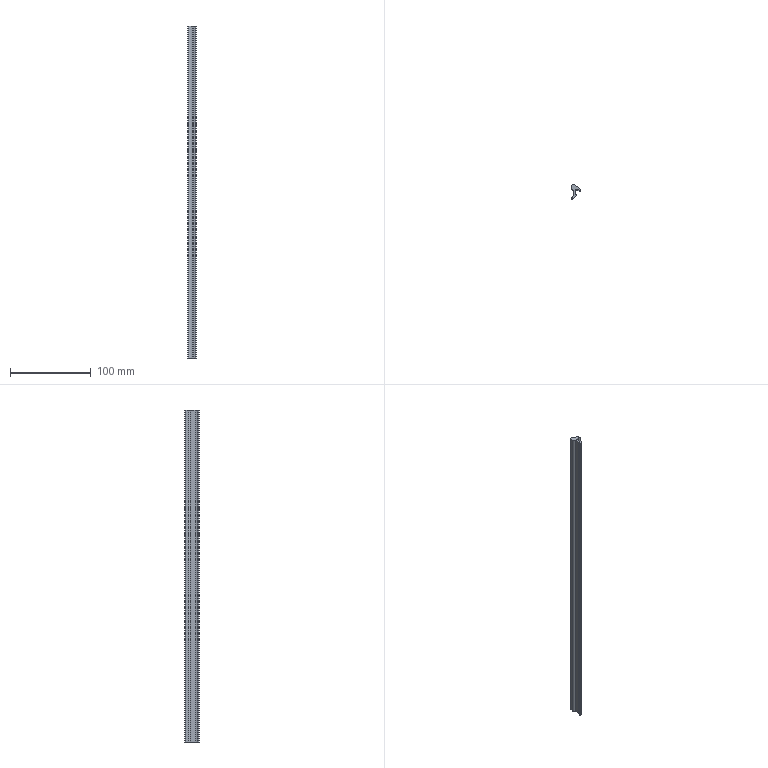Part | SolidWorks | features BaseBody 1, MoveFace 1 | 1 solid | 20 faces | box 10.8 x 17.5 x 410 mm | volume 32308 mm3 | cylinder 11 | plane 9 | commonest cylinder face diameters 1.6 x2 14 x2 0.4 x1 0.6 x1 0.8 x1 2.6 x1
STEP:
#1=CARTESIAN_POINT('',(-3.236,-11.055,310.));
#2=VERTEX_POINT('',#1);
#3=CARTESIAN_POINT('',(-4.3,-10.3,310.));
#4=VERTEX_POINT('',#3);
#5=CARTESIAN_POINT('',(-3.5,-10.3,310.));
#6=DIRECTION('',(0.,0.,-1.));
#7=DIRECTION('',(1.,0.,0.));
#8=AXIS2_PLACEMENT_3D('',#5,#6,#7);
#9=CIRCLE('',#8,0.8);
#10=EDGE_CURVE('',#2,#4,#9,.T.);
#11=ORIENTED_EDGE('',*,*,#10,.T.);
#12=CARTESIAN_POINT('',(-4.3,-10.3,-100.));
#13=VERTEX_POINT('',#12);
#14=CARTESIAN_POINT('',(-4.3,-10.3,-100.));
#15=DIRECTION('',(0.,0.,-1.));
#16=VECTOR('',#15,1000.);
#17=LINE('',#14,#16);
#18=EDGE_CURVE('',#4,#13,#17,.T.);
#19=ORIENTED_EDGE('',*,*,#18,.T.);
#20=CARTESIAN_POINT('',(-3.236,-11.055,-100.));
#21=VERTEX_POINT('',#20);
#22=CARTESIAN_POINT('',(-3.5,-10.3,-100.));
#23=DIRECTION('',(0.,0.,1.));
#24=DIRECTION('',(-1.,0.,0.));
#25=AXIS2_PLACEMENT_3D('',#22,#23,#24);
#26=CIRCLE('',#25,0.8);
#27=EDGE_CURVE('',#13,#21,#26,.T.);
#28=ORIENTED_EDGE('',*,*,#27,.T.);
#29=CARTESIAN_POINT('',(-3.236,-11.055,-100.));
#30=DIRECTION('',(0.,0.,-1.));
#31=VECTOR('',#30,1000.);
#32=LINE('',#29,#31);
#33=EDGE_CURVE('',#2,#21,#32,.T.);
#34=ORIENTED_EDGE('',*,*,#33,.F.);
#35=EDGE_LOOP('',(#11,#19,#28,#34));
#36=FACE_OUTER_BOUND('',#35,.T.);
#37=CARTESIAN_POINT('',(-3.5,-10.3,-100.));
#38=DIRECTION('',(0.,0.,-1.));
#39=DIRECTION('',(-1.,0.,0.));
#40=AXIS2_PLACEMENT_3D('',#37,#38,#39);
#41=CYLINDRICAL_SURFACE('',#40,0.8);
#42=ADVANCED_FACE('',(#36),#41,.T.);
#43=CARTESIAN_POINT('',(1.184,-6.397,-100.));
#44=VERTEX_POINT('',#43);
#45=CARTESIAN_POINT('',(-5.702,-4.29,-100.));
#46=DIRECTION('',(0.,0.,1.));
#47=DIRECTION('',(-1.,0.,0.));
#48=AXIS2_PLACEMENT_3D('',#45,#46,#47);
#49=CIRCLE('',#48,7.201);
#50=EDGE_CURVE('',#21,#44,#49,.T.);
#51=ORIENTED_EDGE('',*,*,#50,.T.);
#52=CARTESIAN_POINT('',(1.184,-6.397,310.));
#53=VERTEX_POINT('',#52);
#54=CARTESIAN_POINT('',(1.184,-6.397,-100.));
#55=DIRECTION('',(0.,0.,1.));
#56=VECTOR('',#55,1000.);
#57=LINE('',#54,#56);
#58=EDGE_CURVE('',#44,#53,#57,.T.);
#59=ORIENTED_EDGE('',*,*,#58,.T.);
#60=CARTESIAN_POINT('',(-5.702,-4.29,310.));
#61=DIRECTION('',(0.,0.,-1.));
#62=DIRECTION('',(1.,0.,0.));
#63=AXIS2_PLACEMENT_3D('',#60,#61,#62);
#64=CIRCLE('',#63,7.201);
#65=EDGE_CURVE('',#53,#2,#64,.T.);
#66=ORIENTED_EDGE('',*,*,#65,.T.);
#67=ORIENTED_EDGE('',*,*,#33,.T.);
#68=EDGE_LOOP('',(#51,#59,#66,#67));
#69=FACE_OUTER_BOUND('',#68,.T.);
#70=CARTESIAN_POINT('',(-5.702,-4.29,-100.));
#71=DIRECTION('',(0.,0.,-1.));
#72=DIRECTION('',(-1.,0.,0.));
#73=AXIS2_PLACEMENT_3D('',#70,#71,#72);
#74=CYLINDRICAL_SURFACE('',#73,7.201);
#75=ADVANCED_FACE('',(#69),#74,.T.);
#76=CARTESIAN_POINT('',(0.9,-6.,-100.));
#77=VERTEX_POINT('',#76);
#78=CARTESIAN_POINT('',(0.9,-6.3,-100.));
#79=DIRECTION('',(0.,0.,1.));
#80=DIRECTION('',(-1.,0.,0.));
#81=AXIS2_PLACEMENT_3D('',#78,#79,#80);
#82=CIRCLE('',#81,0.3);
#83=EDGE_CURVE('',#44,#77,#82,.T.);
#84=ORIENTED_EDGE('',*,*,#83,.T.);
#85=CARTESIAN_POINT('',(0.9,-6.,310.));
#86=VERTEX_POINT('',#85);
#87=CARTESIAN_POINT('',(0.9,-6.,-100.));
#88=DIRECTION('',(0.,0.,1.));
#89=VECTOR('',#88,1000.);
#90=LINE('',#87,#89);
#91=EDGE_CURVE('',#77,#86,#90,.T.);
#92=ORIENTED_EDGE('',*,*,#91,.T.);
#93=CARTESIAN_POINT('',(0.9,-6.3,310.));
#94=DIRECTION('',(0.,0.,-1.));
#95=DIRECTION('',(1.,0.,0.));
#96=AXIS2_PLACEMENT_3D('',#93,#94,#95);
#97=CIRCLE('',#96,0.3);
#98=EDGE_CURVE('',#86,#53,#97,.T.);
#99=ORIENTED_EDGE('',*,*,#98,.T.);
#100=ORIENTED_EDGE('',*,*,#58,.F.);
#101=EDGE_LOOP('',(#84,#92,#99,#100));
#102=FACE_OUTER_BOUND('',#101,.T.);
#103=CARTESIAN_POINT('',(0.9,-6.3,-100.));
#104=DIRECTION('',(0.,0.,-1.));
#105=DIRECTION('',(-1.,0.,0.));
#106=AXIS2_PLACEMENT_3D('',#103,#104,#105);
#107=CYLINDRICAL_SURFACE('',#106,0.3);
#108=ADVANCED_FACE('',(#102),#107,.T.);
#109=CARTESIAN_POINT('',(-2.5,-0.5,-100.));
#110=VERTEX_POINT('',#109);
#111=CARTESIAN_POINT('',(-2.5,-6.153,-100.));
#112=VERTEX_POINT('',#111);
#113=CARTESIAN_POINT('',(-2.5,-6.397,-100.));
#114=DIRECTION('',(0.,-1.,0.));
#115=VECTOR('',#114,1000.);
#116=LINE('',#113,#115);
#117=EDGE_CURVE('',#110,#112,#116,.T.);
#118=ORIENTED_EDGE('',*,*,#117,.F.);
#119=CARTESIAN_POINT('',(-4.2,1.695,-100.));
#120=VERTEX_POINT('',#119);
#121=CARTESIAN_POINT('',(-1.701,1.875,-100.));
#122=DIRECTION('',(0.,0.,1.));
#123=DIRECTION('',(-1.,0.,0.));
#124=AXIS2_PLACEMENT_3D('',#121,#122,#123);
#125=CIRCLE('',#124,2.506);
#126=EDGE_CURVE('',#120,#110,#125,.T.);
#127=ORIENTED_EDGE('',*,*,#126,.F.);
#128=CARTESIAN_POINT('',(-4.2,5.1,-100.));
#129=VERTEX_POINT('',#128);
#130=CARTESIAN_POINT('',(-4.2,-6.397,-100.));
#131=DIRECTION('',(0.,-1.,0.));
#132=VECTOR('',#131,1000.);
#133=LINE('',#130,#132);
#134=EDGE_CURVE('',#129,#120,#133,.T.);
#135=ORIENTED_EDGE('',*,*,#134,.F.);
#136=CARTESIAN_POINT('',(-2.892,6.4,-100.));
#137=VERTEX_POINT('',#136);
#138=CARTESIAN_POINT('',(-2.9,5.1,-100.));
#139=DIRECTION('',(0.,0.,1.));
#140=DIRECTION('',(-1.,0.,0.));
#141=AXIS2_PLACEMENT_3D('',#138,#139,#140);
#142=CIRCLE('',#141,1.3);
#143=EDGE_CURVE('',#137,#129,#142,.T.);
#144=ORIENTED_EDGE('',*,*,#143,.F.);
#145=CARTESIAN_POINT('',(0.5,5.5,-100.));
#146=VERTEX_POINT('',#145);
#147=CARTESIAN_POINT('',(-2.934,-0.5999,-100.));
#148=DIRECTION('',(0.,0.,1.));
#149=DIRECTION('',(-1.,0.,0.));
#150=AXIS2_PLACEMENT_3D('',#147,#148,#149);
#151=CIRCLE('',#150,7.);
#152=EDGE_CURVE('',#146,#137,#151,.T.);
#153=ORIENTED_EDGE('',*,*,#152,.F.);
#154=CARTESIAN_POINT('',(5.5,1.7,-100.));
#155=VERTEX_POINT('',#154);
#156=CARTESIAN_POINT('',(5.5,1.7,-100.));
#157=DIRECTION('',(-0.7962,0.6051,0.));
#158=VECTOR('',#157,1000.);
#159=LINE('',#156,#158);
#160=EDGE_CURVE('',#155,#146,#159,.T.);
#161=ORIENTED_EDGE('',*,*,#160,.F.);
#162=CARTESIAN_POINT('',(6.458,-0.2215,-100.));
#163=VERTEX_POINT('',#162);
#164=CARTESIAN_POINT('',(6.458,-0.2215,-100.));
#165=DIRECTION('',(-0.4462,0.8949,0.));
#166=VECTOR('',#165,1000.);
#167=LINE('',#164,#166);
#168=EDGE_CURVE('',#163,#155,#167,.T.);
#169=ORIENTED_EDGE('',*,*,#168,.F.);
#170=CARTESIAN_POINT('',(5.895,-0.7433,-100.));
#171=VERTEX_POINT('',#170);
#172=CARTESIAN_POINT('',(6.1,-0.4,-100.));
#173=DIRECTION('',(0.,0.,1.));
#174=DIRECTION('',(-1.,0.,0.));
#175=AXIS2_PLACEMENT_3D('',#172,#173,#174);
#176=CIRCLE('',#175,0.4);
#177=EDGE_CURVE('',#171,#163,#176,.T.);
#178=ORIENTED_EDGE('',*,*,#177,.F.);
#179=CARTESIAN_POINT('',(3.,0.,-100.));
#180=VERTEX_POINT('',#179);
#181=CARTESIAN_POINT('',(2.746,-6.995,-100.));
#182=DIRECTION('',(0.,0.,-1.));
#183=DIRECTION('',(-1.,0.,0.));
#184=AXIS2_PLACEMENT_3D('',#181,#182,#183);
#185=CIRCLE('',#184,7.);
#186=EDGE_CURVE('',#180,#171,#185,.T.);
#187=ORIENTED_EDGE('',*,*,#186,.F.);
#188=CARTESIAN_POINT('',(0.,0.,-100.));
#189=VERTEX_POINT('',#188);
#190=CARTESIAN_POINT('',(-6.814,0.,-100.));
#191=DIRECTION('',(1.,0.,0.));
#192=VECTOR('',#191,1000.);
#193=LINE('',#190,#192);
#194=EDGE_CURVE('',#189,#180,#193,.T.);
#195=ORIENTED_EDGE('',*,*,#194,.F.);
#196=CARTESIAN_POINT('',(0.,-5.8,-100.));
#197=VERTEX_POINT('',#196);
#198=CARTESIAN_POINT('',(0.,-6.397,-100.));
#199=DIRECTION('',(0.,1.,0.));
#200=VECTOR('',#199,1000.);
#201=LINE('',#198,#200);
#202=EDGE_CURVE('',#197,#189,#201,.T.);
#203=ORIENTED_EDGE('',*,*,#202,.F.);
#204=CARTESIAN_POINT('',(0.2,-6.,-100.));
#205=VERTEX_POINT('',#204);
#206=CARTESIAN_POINT('',(0.2,-5.8,-100.));
#207=DIRECTION('',(0.,0.,1.));
#208=DIRECTION('',(-1.,0.,0.));
#209=AXIS2_PLACEMENT_3D('',#206,#207,#208);
#210=CIRCLE('',#209,0.2);
#211=EDGE_CURVE('',#197,#205,#210,.T.);
#212=ORIENTED_EDGE('',*,*,#211,.T.);
#213=CARTESIAN_POINT('',(-6.814,-6.,-100.));
#214=DIRECTION('',(-1.,0.,0.));
#215=VECTOR('',#214,1000.);
#216=LINE('',#213,#215);
#217=EDGE_CURVE('',#77,#205,#216,.T.);
#218=ORIENTED_EDGE('',*,*,#217,.F.);
#219=ORIENTED_EDGE('',*,*,#83,.F.);
#220=ORIENTED_EDGE('',*,*,#50,.F.);
#221=ORIENTED_EDGE('',*,*,#27,.F.);
#222=CARTESIAN_POINT('',(-3.998,-9.674,-100.));
#223=VERTEX_POINT('',#222);
#224=CARTESIAN_POINT('',(-3.5,-10.3,-100.));
#225=DIRECTION('',(0.,0.,1.));
#226=DIRECTION('',(-1.,0.,0.));
#227=AXIS2_PLACEMENT_3D('',#224,#225,#226);
#228=CIRCLE('',#227,0.8);
#229=EDGE_CURVE('',#223,#13,#228,.T.);
#230=ORIENTED_EDGE('',*,*,#229,.F.);
#231=CARTESIAN_POINT('',(-6.814,-6.397,-100.));
#232=DIRECTION('',(0.,0.,-1.));
#233=DIRECTION('',(-1.,0.,0.));
#234=AXIS2_PLACEMENT_3D('',#231,#232,#233);
#235=CIRCLE('',#234,4.321);
#236=EDGE_CURVE('',#112,#223,#235,.T.);
#237=ORIENTED_EDGE('',*,*,#236,.F.);
#238=EDGE_LOOP('',(#118,#127,#135,#144,#153,#161,#169,#178,#187,#195,#203,#212,#218,#219,#220,#221,#230,#237));
#239=FACE_OUTER_BOUND('',#238,.T.);
#240=CARTESIAN_POINT('',(-6.814,-6.397,-100.));
#241=DIRECTION('',(0.,0.,1.));
#242=DIRECTION('',(1.,0.,0.));
#243=AXIS2_PLACEMENT_3D('',#240,#241,#242);
#244=PLANE('',#243);
#245=ADVANCED_FACE('',(#239),#244,.F.);
#246=ORIENTED_EDGE('',*,*,#18,.F.);
#247=CARTESIAN_POINT('',(-3.998,-9.674,310.));
#248=VERTEX_POINT('',#247);
#249=CARTESIAN_POINT('',(-3.5,-10.3,310.));
#250=DIRECTION('',(0.,0.,-1.));
#251=DIRECTION('',(1.,0.,0.));
#252=AXIS2_PLACEMENT_3D('',#249,#250,#251);
#253=CIRCLE('',#252,0.8);
#254=EDGE_CURVE('',#4,#248,#253,.T.);
#255=ORIENTED_EDGE('',*,*,#254,.T.);
#256=CARTESIAN_POINT('',(-3.998,-9.674,-100.));
#257=DIRECTION('',(0.,0.,-1.));
#258=VECTOR('',#257,1000.);
#259=LINE('',#256,#258);
#260=EDGE_CURVE('',#248,#223,#259,.T.);
#261=ORIENTED_EDGE('',*,*,#260,.T.);
#262=ORIENTED_EDGE('',*,*,#229,.T.);
#263=EDGE_LOOP('',(#246,#255,#261,#262));
#264=FACE_OUTER_BOUND('',#263,.T.);
#265=CARTESIAN_POINT('',(-3.5,-10.3,-100.));
#266=DIRECTION('',(0.,0.,-1.));
#267=DIRECTION('',(-1.,0.,0.));
#268=AXIS2_PLACEMENT_3D('',#265,#266,#267);
#269=CYLINDRICAL_SURFACE('',#268,0.8);
#270=ADVANCED_FACE('',(#264),#269,.T.);
#271=CARTESIAN_POINT('',(-4.2,1.695,310.));
#272=VERTEX_POINT('',#271);
#273=CARTESIAN_POINT('',(-2.5,-0.5,310.));
#274=VERTEX_POINT('',#273);
#275=CARTESIAN_POINT('',(-1.701,1.875,310.));
#276=DIRECTION('',(0.,0.,1.));
#277=DIRECTION('',(1.,0.,0.));
#278=AXIS2_PLACEMENT_3D('',#275,#276,#277);
#279=CIRCLE('',#278,2.506);
#280=EDGE_CURVE('',#272,#274,#279,.T.);
#281=ORIENTED_EDGE('',*,*,#280,.T.);
#282=CARTESIAN_POINT('',(-2.5,-6.153,310.));
#283=VERTEX_POINT('',#282);
#284=CARTESIAN_POINT('',(-2.5,-6.397,310.));
#285=DIRECTION('',(0.,-1.,0.));
#286=VECTOR('',#285,1000.);
#287=LINE('',#284,#286);
#288=EDGE_CURVE('',#274,#283,#287,.T.);
#289=ORIENTED_EDGE('',*,*,#288,.T.);
#290=CARTESIAN_POINT('',(-6.814,-6.397,310.));
#291=DIRECTION('',(0.,0.,-1.));
#292=DIRECTION('',(1.,0.,0.));
#293=AXIS2_PLACEMENT_3D('',#290,#291,#292);
#294=CIRCLE('',#293,4.321);
#295=EDGE_CURVE('',#283,#248,#294,.T.);
#296=ORIENTED_EDGE('',*,*,#295,.T.);
#297=ORIENTED_EDGE('',*,*,#254,.F.);
#298=ORIENTED_EDGE('',*,*,#10,.F.);
#299=ORIENTED_EDGE('',*,*,#65,.F.);
#300=ORIENTED_EDGE('',*,*,#98,.F.);
#301=CARTESIAN_POINT('',(0.2,-6.,310.));
#302=VERTEX_POINT('',#301);
#303=CARTESIAN_POINT('',(-6.814,-6.,310.));
#304=DIRECTION('',(-1.,0.,0.));
#305=VECTOR('',#304,1000.);
#306=LINE('',#303,#305);
#307=EDGE_CURVE('',#86,#302,#306,.T.);
#308=ORIENTED_EDGE('',*,*,#307,.T.);
#309=CARTESIAN_POINT('',(0.,-5.8,310.));
#310=VERTEX_POINT('',#309);
#311=CARTESIAN_POINT('',(0.2,-5.8,310.));
#312=DIRECTION('',(0.,0.,-1.));
#313=DIRECTION('',(1.,0.,0.));
#314=AXIS2_PLACEMENT_3D('',#311,#312,#313);
#315=CIRCLE('',#314,0.2);
#316=EDGE_CURVE('',#302,#310,#315,.T.);
#317=ORIENTED_EDGE('',*,*,#316,.T.);
#318=CARTESIAN_POINT('',(0.,0.,310.));
#319=VERTEX_POINT('',#318);
#320=CARTESIAN_POINT('',(0.,-6.397,310.));
#321=DIRECTION('',(0.,1.,0.));
#322=VECTOR('',#321,1000.);
#323=LINE('',#320,#322);
#324=EDGE_CURVE('',#310,#319,#323,.T.);
#325=ORIENTED_EDGE('',*,*,#324,.T.);
#326=CARTESIAN_POINT('',(3.,0.,310.));
#327=VERTEX_POINT('',#326);
#328=CARTESIAN_POINT('',(-6.814,0.,310.));
#329=DIRECTION('',(1.,0.,0.));
#330=VECTOR('',#329,1000.);
#331=LINE('',#328,#330);
#332=EDGE_CURVE('',#319,#327,#331,.T.);
#333=ORIENTED_EDGE('',*,*,#332,.T.);
#334=CARTESIAN_POINT('',(5.895,-0.7433,310.));
#335=VERTEX_POINT('',#334);
#336=CARTESIAN_POINT('',(2.746,-6.995,310.));
#337=DIRECTION('',(0.,0.,-1.));
#338=DIRECTION('',(1.,0.,0.));
#339=AXIS2_PLACEMENT_3D('',#336,#337,#338);
#340=CIRCLE('',#339,7.);
#341=EDGE_CURVE('',#327,#335,#340,.T.);
#342=ORIENTED_EDGE('',*,*,#341,.T.);
#343=CARTESIAN_POINT('',(6.458,-0.2215,310.));
#344=VERTEX_POINT('',#343);
#345=CARTESIAN_POINT('',(6.1,-0.4,310.));
#346=DIRECTION('',(0.,0.,-1.));
#347=DIRECTION('',(1.,0.,0.));
#348=AXIS2_PLACEMENT_3D('',#345,#346,#347);
#349=CIRCLE('',#348,0.4);
#350=EDGE_CURVE('',#344,#335,#349,.T.);
#351=ORIENTED_EDGE('',*,*,#350,.F.);
#352=CARTESIAN_POINT('',(5.5,1.7,310.));
#353=VERTEX_POINT('',#352);
#354=CARTESIAN_POINT('',(6.282,0.1323,310.));
#355=DIRECTION('',(-0.4462,0.8949,0.));
#356=VECTOR('',#355,1000.);
#357=LINE('',#354,#356);
#358=EDGE_CURVE('',#344,#353,#357,.T.);
#359=ORIENTED_EDGE('',*,*,#358,.T.);
#360=CARTESIAN_POINT('',(0.5,5.5,310.));
#361=VERTEX_POINT('',#360);
#362=CARTESIAN_POINT('',(1.595,4.668,310.));
#363=DIRECTION('',(-0.7962,0.6051,0.));
#364=VECTOR('',#363,1000.);
#365=LINE('',#362,#364);
#366=EDGE_CURVE('',#353,#361,#365,.T.);
#367=ORIENTED_EDGE('',*,*,#366,.T.);
#368=CARTESIAN_POINT('',(-2.892,6.4,310.));
#369=VERTEX_POINT('',#368);
#370=CARTESIAN_POINT('',(-2.934,-0.5999,310.));
#371=DIRECTION('',(0.,0.,1.));
#372=DIRECTION('',(1.,0.,0.));
#373=AXIS2_PLACEMENT_3D('',#370,#371,#372);
#374=CIRCLE('',#373,7.);
#375=EDGE_CURVE('',#361,#369,#374,.T.);
#376=ORIENTED_EDGE('',*,*,#375,.T.);
#377=CARTESIAN_POINT('',(-4.2,5.1,310.));
#378=VERTEX_POINT('',#377);
#379=CARTESIAN_POINT('',(-2.9,5.1,310.));
#380=DIRECTION('',(0.,0.,1.));
#381=DIRECTION('',(1.,0.,0.));
#382=AXIS2_PLACEMENT_3D('',#379,#380,#381);
#383=CIRCLE('',#382,1.3);
#384=EDGE_CURVE('',#369,#378,#383,.T.);
#385=ORIENTED_EDGE('',*,*,#384,.T.);
#386=CARTESIAN_POINT('',(-4.2,-6.397,310.));
#387=DIRECTION('',(0.,-1.,0.));
#388=VECTOR('',#387,1000.);
#389=LINE('',#386,#388);
#390=EDGE_CURVE('',#378,#272,#389,.T.);
#391=ORIENTED_EDGE('',*,*,#390,.T.);
#392=EDGE_LOOP('',(#281,#289,#296,#297,#298,#299,#300,#308,#317,#325,#333,#342,#351,#359,#367,#376,#385,#391));
#393=FACE_OUTER_BOUND('',#392,.T.);
#394=CARTESIAN_POINT('',(-6.814,-6.397,310.));
#395=DIRECTION('',(0.,0.,1.));
#396=DIRECTION('',(1.,0.,0.));
#397=AXIS2_PLACEMENT_3D('',#394,#395,#396);
#398=PLANE('',#397);
#399=ADVANCED_FACE('',(#393),#398,.T.);
#400=ORIENTED_EDGE('',*,*,#217,.T.);
#401=CARTESIAN_POINT('',(0.2,-6.,-100.));
#402=DIRECTION('',(0.,0.,1.));
#403=VECTOR('',#402,1000.);
#404=LINE('',#401,#403);
#405=EDGE_CURVE('',#205,#302,#404,.T.);
#406=ORIENTED_EDGE('',*,*,#405,.T.);
#407=ORIENTED_EDGE('',*,*,#307,.F.);
#408=ORIENTED_EDGE('',*,*,#91,.F.);
#409=EDGE_LOOP('',(#400,#406,#407,#408));
#410=FACE_OUTER_BOUND('',#409,.T.);
#411=CARTESIAN_POINT('',(0.9,-6.,-100.));
#412=DIRECTION('',(0.,1.,0.));
#413=DIRECTION('',(0.,0.,1.));
#414=AXIS2_PLACEMENT_3D('',#411,#412,#413);
#415=PLANE('',#414);
#416=ADVANCED_FACE('',(#410),#415,.T.);
#417=CARTESIAN_POINT('',(-2.5,-6.153,-100.));
#418=DIRECTION('',(0.,0.,1.));
#419=VECTOR('',#418,1000.);
#420=LINE('',#417,#419);
#421=EDGE_CURVE('',#112,#283,#420,.T.);
#422=ORIENTED_EDGE('',*,*,#421,.F.);
#423=ORIENTED_EDGE('',*,*,#236,.T.);
#424=ORIENTED_EDGE('',*,*,#260,.F.);
#425=ORIENTED_EDGE('',*,*,#295,.F.);
#426=EDGE_LOOP('',(#422,#423,#424,#425));
#427=FACE_OUTER_BOUND('',#426,.T.);
#428=CARTESIAN_POINT('',(-6.814,-6.397,-100.));
#429=DIRECTION('',(0.,0.,-1.));
#430=DIRECTION('',(-1.,0.,0.));
#431=AXIS2_PLACEMENT_3D('',#428,#429,#430);
#432=CYLINDRICAL_SURFACE('',#431,4.321);
#433=ADVANCED_FACE('',(#427),#432,.F.);
#434=ORIENTED_EDGE('',*,*,#117,.T.);
#435=ORIENTED_EDGE('',*,*,#421,.T.);
#436=ORIENTED_EDGE('',*,*,#288,.F.);
#437=CARTESIAN_POINT('',(-2.5,-0.5,-100.));
#438=DIRECTION('',(0.,0.,-1.));
#439=VECTOR('',#438,1000.);
#440=LINE('',#437,#439);
#441=EDGE_CURVE('',#274,#110,#440,.T.);
#442=ORIENTED_EDGE('',*,*,#441,.T.);
#443=EDGE_LOOP('',(#434,#435,#436,#442));
#444=FACE_OUTER_BOUND('',#443,.T.);
#445=CARTESIAN_POINT('',(-2.5,-0.5,-100.));
#446=DIRECTION('',(-1.,0.,0.));
#447=DIRECTION('',(0.,0.,1.));
#448=AXIS2_PLACEMENT_3D('',#445,#446,#447);
#449=PLANE('',#448);
#450=ADVANCED_FACE('',(#444),#449,.T.);
#451=ORIENTED_EDGE('',*,*,#126,.T.);
#452=ORIENTED_EDGE('',*,*,#441,.F.);
#453=ORIENTED_EDGE('',*,*,#280,.F.);
#454=CARTESIAN_POINT('',(-4.2,1.695,-100.));
#455=DIRECTION('',(0.,0.,-1.));
#456=VECTOR('',#455,1000.);
#457=LINE('',#454,#456);
#458=EDGE_CURVE('',#272,#120,#457,.T.);
#459=ORIENTED_EDGE('',*,*,#458,.T.);
#460=EDGE_LOOP('',(#451,#452,#453,#459));
#461=FACE_OUTER_BOUND('',#460,.T.);
#462=CARTESIAN_POINT('',(-1.701,1.875,-100.));
#463=DIRECTION('',(0.,0.,-1.));
#464=DIRECTION('',(-1.,0.,0.));
#465=AXIS2_PLACEMENT_3D('',#462,#463,#464);
#466=CYLINDRICAL_SURFACE('',#465,2.506);
#467=ADVANCED_FACE('',(#461),#466,.T.);
#468=ORIENTED_EDGE('',*,*,#134,.T.);
#469=ORIENTED_EDGE('',*,*,#458,.F.);
#470=ORIENTED_EDGE('',*,*,#390,.F.);
#471=CARTESIAN_POINT('',(-4.2,5.1,-100.));
#472=DIRECTION('',(0.,0.,-1.));
#473=VECTOR('',#472,1000.);
#474=LINE('',#471,#473);
#475=EDGE_CURVE('',#378,#129,#474,.T.);
#476=ORIENTED_EDGE('',*,*,#475,.T.);
#477=EDGE_LOOP('',(#468,#469,#470,#476));
#478=FACE_OUTER_BOUND('',#477,.T.);
#479=CARTESIAN_POINT('',(-4.2,5.1,-100.));
#480=DIRECTION('',(-1.,0.,0.));
#481=DIRECTION('',(0.,0.,1.));
#482=AXIS2_PLACEMENT_3D('',#479,#480,#481);
#483=PLANE('',#482);
#484=ADVANCED_FACE('',(#478),#483,.T.);
#485=ORIENTED_EDGE('',*,*,#143,.T.);
#486=ORIENTED_EDGE('',*,*,#475,.F.);
#487=ORIENTED_EDGE('',*,*,#384,.F.);
#488=CARTESIAN_POINT('',(-2.892,6.4,-100.));
#489=DIRECTION('',(0.,0.,-1.));
#490=VECTOR('',#489,1000.);
#491=LINE('',#488,#490);
#492=EDGE_CURVE('',#369,#137,#491,.T.);
#493=ORIENTED_EDGE('',*,*,#492,.T.);
#494=EDGE_LOOP('',(#485,#486,#487,#493));
#495=FACE_OUTER_BOUND('',#494,.T.);
#496=CARTESIAN_POINT('',(-2.9,5.1,-100.));
#497=DIRECTION('',(0.,0.,-1.));
#498=DIRECTION('',(-1.,0.,0.));
#499=AXIS2_PLACEMENT_3D('',#496,#497,#498);
#500=CYLINDRICAL_SURFACE('',#499,1.3);
#501=ADVANCED_FACE('',(#495),#500,.T.);
#502=ORIENTED_EDGE('',*,*,#152,.T.);
#503=ORIENTED_EDGE('',*,*,#492,.F.);
#504=ORIENTED_EDGE('',*,*,#375,.F.);
#505=CARTESIAN_POINT('',(0.5,5.5,-100.));
#506=DIRECTION('',(0.,0.,-1.));
#507=VECTOR('',#506,1000.);
#508=LINE('',#505,#507);
#509=EDGE_CURVE('',#361,#146,#508,.T.);
#510=ORIENTED_EDGE('',*,*,#509,.T.);
#511=EDGE_LOOP('',(#502,#503,#504,#510));
#512=FACE_OUTER_BOUND('',#511,.T.);
#513=CARTESIAN_POINT('',(-2.934,-0.5999,-100.));
#514=DIRECTION('',(0.,0.,-1.));
#515=DIRECTION('',(-1.,0.,0.));
#516=AXIS2_PLACEMENT_3D('',#513,#514,#515);
#517=CYLINDRICAL_SURFACE('',#516,7.);
#518=ADVANCED_FACE('',(#512),#517,.T.);
#519=ORIENTED_EDGE('',*,*,#160,.T.);
#520=ORIENTED_EDGE('',*,*,#509,.F.);
#521=ORIENTED_EDGE('',*,*,#366,.F.);
#522=CARTESIAN_POINT('',(5.5,1.7,-100.));
#523=DIRECTION('',(0.,0.,-1.));
#524=VECTOR('',#523,1000.);
#525=LINE('',#522,#524);
#526=EDGE_CURVE('',#353,#155,#525,.T.);
#527=ORIENTED_EDGE('',*,*,#526,.T.);
#528=EDGE_LOOP('',(#519,#520,#521,#527));
#529=FACE_OUTER_BOUND('',#528,.T.);
#530=CARTESIAN_POINT('',(5.5,1.7,-100.));
#531=DIRECTION('',(0.6051,0.7962,0.));
#532=DIRECTION('',(-0.7962,0.6051,0.));
#533=AXIS2_PLACEMENT_3D('',#530,#531,#532);
#534=PLANE('',#533);
#535=ADVANCED_FACE('',(#529),#534,.T.);
#536=ORIENTED_EDGE('',*,*,#168,.T.);
#537=ORIENTED_EDGE('',*,*,#526,.F.);
#538=ORIENTED_EDGE('',*,*,#358,.F.);
#539=CARTESIAN_POINT('',(6.458,-0.2215,-100.));
#540=DIRECTION('',(0.,0.,-1.));
#541=VECTOR('',#540,1000.);
#542=LINE('',#539,#541);
#543=EDGE_CURVE('',#344,#163,#542,.T.);
#544=ORIENTED_EDGE('',*,*,#543,.T.);
#545=EDGE_LOOP('',(#536,#537,#538,#544));
#546=FACE_OUTER_BOUND('',#545,.T.);
#547=CARTESIAN_POINT('',(6.458,-0.2215,-100.));
#548=DIRECTION('',(0.8949,0.4462,0.));
#549=DIRECTION('',(-0.4462,0.8949,0.));
#550=AXIS2_PLACEMENT_3D('',#547,#548,#549);
#551=PLANE('',#550);
#552=ADVANCED_FACE('',(#546),#551,.T.);
#553=CARTESIAN_POINT('',(3.,0.,-100.));
#554=DIRECTION('',(0.,0.,1.));
#555=VECTOR('',#554,1000.);
#556=LINE('',#553,#555);
#557=EDGE_CURVE('',#180,#327,#556,.T.);
#558=ORIENTED_EDGE('',*,*,#557,.F.);
#559=ORIENTED_EDGE('',*,*,#186,.T.);
#560=CARTESIAN_POINT('',(5.895,-0.7433,-100.));
#561=DIRECTION('',(0.,0.,-1.));
#562=VECTOR('',#561,1000.);
#563=LINE('',#560,#562);
#564=EDGE_CURVE('',#335,#171,#563,.T.);
#565=ORIENTED_EDGE('',*,*,#564,.F.);
#566=ORIENTED_EDGE('',*,*,#341,.F.);
#567=EDGE_LOOP('',(#558,#559,#565,#566));
#568=FACE_OUTER_BOUND('',#567,.T.);
#569=CARTESIAN_POINT('',(2.746,-6.995,-100.));
#570=DIRECTION('',(0.,0.,-1.));
#571=DIRECTION('',(-1.,0.,0.));
#572=AXIS2_PLACEMENT_3D('',#569,#570,#571);
#573=CYLINDRICAL_SURFACE('',#572,7.);
#574=ADVANCED_FACE('',(#568),#573,.F.);
#575=ORIENTED_EDGE('',*,*,#194,.T.);
#576=ORIENTED_EDGE('',*,*,#557,.T.);
#577=ORIENTED_EDGE('',*,*,#332,.F.);
#578=CARTESIAN_POINT('',(0.,0.,-100.));
#579=DIRECTION('',(0.,0.,-1.));
#580=VECTOR('',#579,1000.);
#581=LINE('',#578,#580);
#582=EDGE_CURVE('',#319,#189,#581,.T.);
#583=ORIENTED_EDGE('',*,*,#582,.T.);
#584=EDGE_LOOP('',(#575,#576,#577,#583));
#585=FACE_OUTER_BOUND('',#584,.T.);
#586=CARTESIAN_POINT('',(0.,0.,-100.));
#587=DIRECTION('',(0.,-1.,0.));
#588=DIRECTION('',(0.,0.,-1.));
#589=AXIS2_PLACEMENT_3D('',#586,#587,#588);
#590=PLANE('',#589);
#591=ADVANCED_FACE('',(#585),#590,.T.);
#592=ORIENTED_EDGE('',*,*,#202,.T.);
#593=ORIENTED_EDGE('',*,*,#582,.F.);
#594=ORIENTED_EDGE('',*,*,#324,.F.);
#595=CARTESIAN_POINT('',(0.,-5.8,-100.));
#596=DIRECTION('',(0.,0.,-1.));
#597=VECTOR('',#596,1000.);
#598=LINE('',#595,#597);
#599=EDGE_CURVE('',#310,#197,#598,.T.);
#600=ORIENTED_EDGE('',*,*,#599,.T.);
#601=EDGE_LOOP('',(#592,#593,#594,#600));
#602=FACE_OUTER_BOUND('',#601,.T.);
#603=CARTESIAN_POINT('',(0.,-5.8,-100.));
#604=DIRECTION('',(1.,0.,0.));
#605=DIRECTION('',(0.,0.,-1.));
#606=AXIS2_PLACEMENT_3D('',#603,#604,#605);
#607=PLANE('',#606);
#608=ADVANCED_FACE('',(#602),#607,.T.);
#609=ORIENTED_EDGE('',*,*,#405,.F.);
#610=ORIENTED_EDGE('',*,*,#211,.F.);
#611=ORIENTED_EDGE('',*,*,#599,.F.);
#612=ORIENTED_EDGE('',*,*,#316,.F.);
#613=EDGE_LOOP('',(#609,#610,#611,#612));
#614=FACE_OUTER_BOUND('',#613,.T.);
#615=CARTESIAN_POINT('',(0.2,-5.8,-100.));
#616=DIRECTION('',(0.,0.,-1.));
#617=DIRECTION('',(-1.,0.,0.));
#618=AXIS2_PLACEMENT_3D('',#615,#616,#617);
#619=CYLINDRICAL_SURFACE('',#618,0.2);
#620=ADVANCED_FACE('',(#614),#619,.F.);
#621=ORIENTED_EDGE('',*,*,#177,.T.);
#622=ORIENTED_EDGE('',*,*,#543,.F.);
#623=ORIENTED_EDGE('',*,*,#350,.T.);
#624=ORIENTED_EDGE('',*,*,#564,.T.);
#625=EDGE_LOOP('',(#621,#622,#623,#624));
#626=FACE_OUTER_BOUND('',#625,.T.);
#627=CARTESIAN_POINT('',(6.1,-0.4,-100.));
#628=DIRECTION('',(0.,0.,-1.));
#629=DIRECTION('',(-1.,0.,0.));
#630=AXIS2_PLACEMENT_3D('',#627,#628,#629);
#631=CYLINDRICAL_SURFACE('',#630,0.4);
#632=ADVANCED_FACE('',(#626),#631,.T.);
#633=CLOSED_SHELL('',(#42,#75,#108,#245,#270,#399,#416,#433,#450,#467,#484,#501,#518,#535,#552,#574,#591,#608,#620,#632));
#634=MANIFOLD_SOLID_BREP('',#633);
#635=CARTESIAN_POINT('',(0.,0.,0.));
#636=DIRECTION('',(0.,0.,1.));
#637=DIRECTION('',(1.,0.,0.));
#638=AXIS2_PLACEMENT_3D('',#635,#636,#637);
#639=(LENGTH_UNIT()NAMED_UNIT(*)SI_UNIT(.MILLI.,.METRE.));
#640=UNCERTAINTY_MEASURE_WITH_UNIT(LENGTH_MEASURE(0.00001),#639,'','');
#641=(NAMED_UNIT(*)PLANE_ANGLE_UNIT()SI_UNIT($,.RADIAN.));
#642=(NAMED_UNIT(*)SI_UNIT($,.STERADIAN.)SOLID_ANGLE_UNIT());
#643=(GEOMETRIC_REPRESENTATION_CONTEXT(3)GLOBAL_UNCERTAINTY_ASSIGNED_CONTEXT((#640))GLOBAL_UNIT_ASSIGNED_CONTEXT((#639,#641,#642))REPRESENTATION_CONTEXT('',''));
#644=ADVANCED_BREP_SHAPE_REPRESENTATION('',(#634,#638),#643);